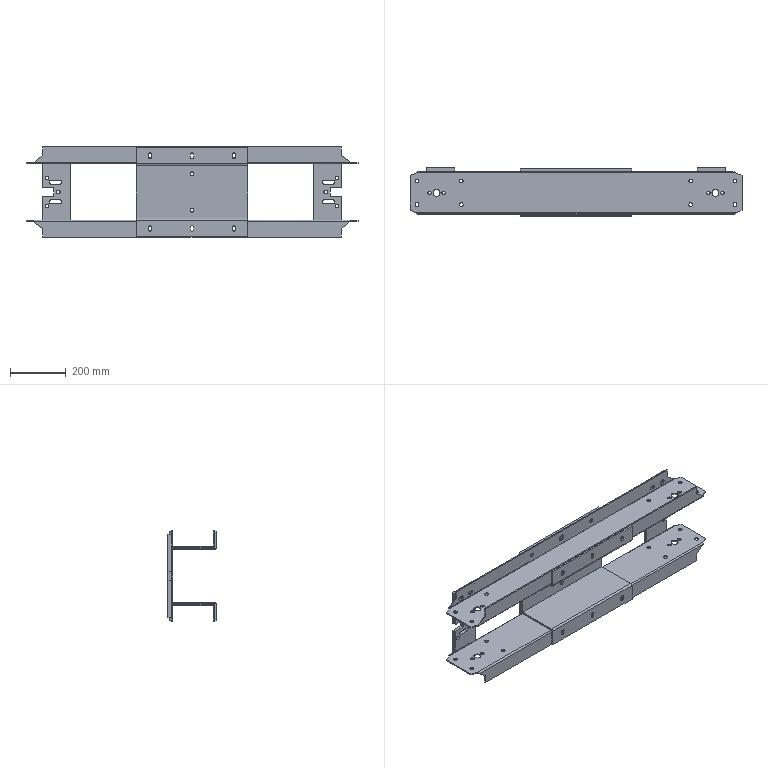Part | 6 solids | 362 faces | box 1186 x 172 x 322 mm | volume 5463825 mm3 | cylinder 194 | plane 160 | spline 8 | commonest cylinder face diameters 14 x142 12 x16 22 x12 25 x8 0.4 x4 2 x4